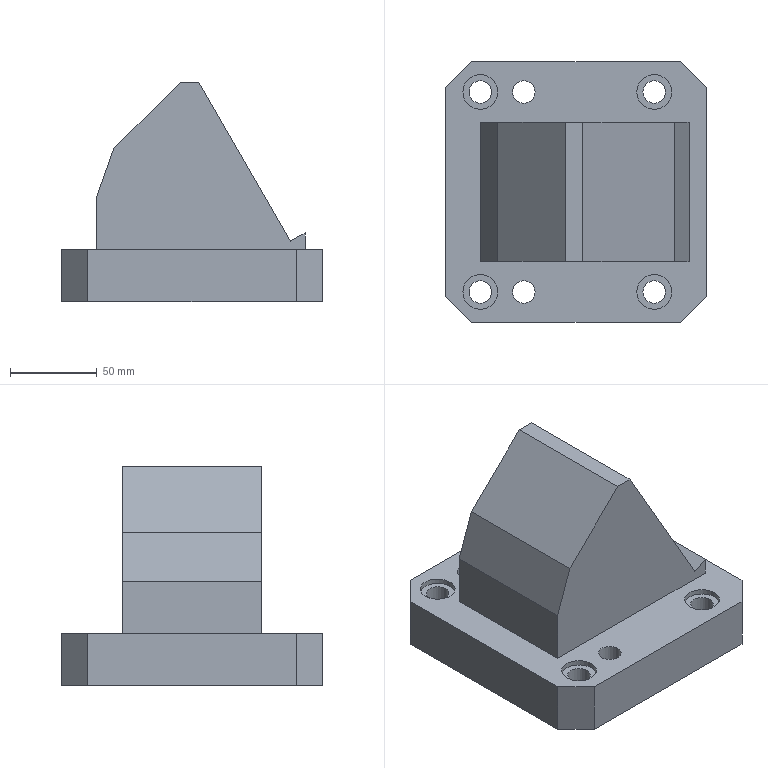Part | NX | features solid 2 | 1 solid | 42 faces | box 150 x 150 x 126.504 mm | volume 1190810 mm3 | plane 32 | cylinder 10 | commonest cylinder face diameters 13 x6 20 x4
STEP:
#1=CARTESIAN_POINT('',(5.,782.5,185.));
#2=VERTEX_POINT('',#1);
#3=CARTESIAN_POINT('',(-5.,782.5,185.));
#4=DIRECTION('',(0.,0.,1.));
#5=DIRECTION('',(1.,0.,0.));
#6=AXIS2_PLACEMENT_3D('',#3,#4,#5);
#7=CIRCLE('',#6,10.);
#8=EDGE_CURVE('',#2,#2,#7,.T.);
#9=ORIENTED_EDGE('',*,*,#8,.F.);
#10=EDGE_LOOP('',(#9));
#11=FACE_BOUND('',#10,.T.);
#12=CARTESIAN_POINT('',(-73.5,782.5,185.));
#13=VERTEX_POINT('',#12);
#14=CARTESIAN_POINT('',(-80.,782.5,185.));
#15=DIRECTION('',(0.,0.,1.));
#16=DIRECTION('',(1.,0.,0.));
#17=AXIS2_PLACEMENT_3D('',#14,#15,#16);
#18=CIRCLE('',#17,6.5);
#19=EDGE_CURVE('',#13,#13,#18,.T.);
#20=ORIENTED_EDGE('',*,*,#19,.F.);
#21=EDGE_LOOP('',(#20));
#22=FACE_BOUND('',#21,.T.);
#23=CARTESIAN_POINT('',(-95.,782.5,185.));
#24=VERTEX_POINT('',#23);
#25=CARTESIAN_POINT('',(-105.,782.5,185.));
#26=DIRECTION('',(0.,0.,1.));
#27=DIRECTION('',(1.,0.,0.));
#28=AXIS2_PLACEMENT_3D('',#25,#26,#27);
#29=CIRCLE('',#28,10.);
#30=EDGE_CURVE('',#24,#24,#29,.T.);
#31=ORIENTED_EDGE('',*,*,#30,.F.);
#32=EDGE_LOOP('',(#31));
#33=FACE_BOUND('',#32,.T.);
#34=CARTESIAN_POINT('',(-95.,667.5,185.));
#35=VERTEX_POINT('',#34);
#36=CARTESIAN_POINT('',(-105.,667.5,185.));
#37=DIRECTION('',(0.,0.,1.));
#38=DIRECTION('',(1.,0.,0.));
#39=AXIS2_PLACEMENT_3D('',#36,#37,#38);
#40=CIRCLE('',#39,10.);
#41=EDGE_CURVE('',#35,#35,#40,.T.);
#42=ORIENTED_EDGE('',*,*,#41,.F.);
#43=EDGE_LOOP('',(#42));
#44=FACE_BOUND('',#43,.T.);
#45=CARTESIAN_POINT('',(-73.5,667.5,185.));
#46=VERTEX_POINT('',#45);
#47=CARTESIAN_POINT('',(-80.,667.5,185.));
#48=DIRECTION('',(0.,0.,1.));
#49=DIRECTION('',(1.,0.,0.));
#50=AXIS2_PLACEMENT_3D('',#47,#48,#49);
#51=CIRCLE('',#50,6.5);
#52=EDGE_CURVE('',#46,#46,#51,.T.);
#53=ORIENTED_EDGE('',*,*,#52,.F.);
#54=EDGE_LOOP('',(#53));
#55=FACE_BOUND('',#54,.T.);
#56=CARTESIAN_POINT('',(5.,667.5,185.));
#57=VERTEX_POINT('',#56);
#58=CARTESIAN_POINT('',(-5.,667.5,185.));
#59=DIRECTION('',(0.,0.,1.));
#60=DIRECTION('',(1.,0.,0.));
#61=AXIS2_PLACEMENT_3D('',#58,#59,#60);
#62=CIRCLE('',#61,10.);
#63=EDGE_CURVE('',#57,#57,#62,.T.);
#64=ORIENTED_EDGE('',*,*,#63,.F.);
#65=EDGE_LOOP('',(#64));
#66=FACE_BOUND('',#65,.T.);
#67=CARTESIAN_POINT('',(-105.,685.,185.));
#68=VERTEX_POINT('',#67);
#69=CARTESIAN_POINT('',(15.,685.,185.));
#70=VERTEX_POINT('',#69);
#71=CARTESIAN_POINT('',(-125.,685.,185.));
#72=DIRECTION('',(1.,0.,0.));
#73=VECTOR('',#72,1000.);
#74=LINE('',#71,#73);
#75=EDGE_CURVE('',#68,#70,#74,.T.);
#76=ORIENTED_EDGE('',*,*,#75,.F.);
#77=CARTESIAN_POINT('',(-105.,765.,185.));
#78=VERTEX_POINT('',#77);
#79=CARTESIAN_POINT('',(-105.,685.,185.));
#80=DIRECTION('',(0.,1.,0.));
#81=VECTOR('',#80,1000.);
#82=LINE('',#79,#81);
#83=EDGE_CURVE('',#68,#78,#82,.T.);
#84=ORIENTED_EDGE('',*,*,#83,.T.);
#85=CARTESIAN_POINT('',(15.,765.,185.));
#86=VERTEX_POINT('',#85);
#87=CARTESIAN_POINT('',(-125.,765.,185.));
#88=DIRECTION('',(1.,0.,0.));
#89=VECTOR('',#88,1000.);
#90=LINE('',#87,#89);
#91=EDGE_CURVE('',#78,#86,#90,.T.);
#92=ORIENTED_EDGE('',*,*,#91,.T.);
#93=CARTESIAN_POINT('',(15.,685.,185.));
#94=DIRECTION('',(0.,1.,0.));
#95=VECTOR('',#94,1000.);
#96=LINE('',#93,#95);
#97=EDGE_CURVE('',#70,#86,#96,.T.);
#98=ORIENTED_EDGE('',*,*,#97,.F.);
#99=EDGE_LOOP('',(#76,#84,#92,#98));
#100=FACE_BOUND('',#99,.T.);
#101=CARTESIAN_POINT('',(-110.,800.,185.));
#102=VERTEX_POINT('',#101);
#103=CARTESIAN_POINT('',(10.,800.,185.));
#104=VERTEX_POINT('',#103);
#105=CARTESIAN_POINT('',(-125.,800.,185.));
#106=DIRECTION('',(1.,0.,0.));
#107=VECTOR('',#106,1000.);
#108=LINE('',#105,#107);
#109=EDGE_CURVE('',#102,#104,#108,.T.);
#110=ORIENTED_EDGE('',*,*,#109,.F.);
#111=CARTESIAN_POINT('',(-125.,785.,185.));
#112=VERTEX_POINT('',#111);
#113=CARTESIAN_POINT('',(-192.5,717.5,185.));
#114=DIRECTION('',(-0.7071,-0.7071,0.));
#115=VECTOR('',#114,1000.);
#116=LINE('',#113,#115);
#117=EDGE_CURVE('',#102,#112,#116,.T.);
#118=ORIENTED_EDGE('',*,*,#117,.T.);
#119=CARTESIAN_POINT('',(-125.,665.,185.));
#120=VERTEX_POINT('',#119);
#121=CARTESIAN_POINT('',(-125.,650.,185.));
#122=DIRECTION('',(0.,1.,0.));
#123=VECTOR('',#122,1000.);
#124=LINE('',#121,#123);
#125=EDGE_CURVE('',#120,#112,#124,.T.);
#126=ORIENTED_EDGE('',*,*,#125,.F.);
#127=CARTESIAN_POINT('',(-110.,650.,185.));
#128=VERTEX_POINT('',#127);
#129=CARTESIAN_POINT('',(-117.5,657.5,185.));
#130=DIRECTION('',(-0.7071,0.7071,0.));
#131=VECTOR('',#130,1000.);
#132=LINE('',#129,#131);
#133=EDGE_CURVE('',#120,#128,#132,.F.);
#134=ORIENTED_EDGE('',*,*,#133,.T.);
#135=CARTESIAN_POINT('',(10.,650.,185.));
#136=VERTEX_POINT('',#135);
#137=CARTESIAN_POINT('',(-125.,650.,185.));
#138=DIRECTION('',(1.,0.,0.));
#139=VECTOR('',#138,1000.);
#140=LINE('',#137,#139);
#141=EDGE_CURVE('',#128,#136,#140,.T.);
#142=ORIENTED_EDGE('',*,*,#141,.T.);
#143=CARTESIAN_POINT('',(25.,665.,185.));
#144=VERTEX_POINT('',#143);
#145=CARTESIAN_POINT('',(-57.5,582.5,185.));
#146=DIRECTION('',(0.7071,0.7071,0.));
#147=VECTOR('',#146,1000.);
#148=LINE('',#145,#147);
#149=EDGE_CURVE('',#136,#144,#148,.T.);
#150=ORIENTED_EDGE('',*,*,#149,.T.);
#151=CARTESIAN_POINT('',(25.,785.,185.));
#152=VERTEX_POINT('',#151);
#153=CARTESIAN_POINT('',(25.,650.,185.));
#154=DIRECTION('',(0.,1.,0.));
#155=VECTOR('',#154,1000.);
#156=LINE('',#153,#155);
#157=EDGE_CURVE('',#144,#152,#156,.T.);
#158=ORIENTED_EDGE('',*,*,#157,.T.);
#159=CARTESIAN_POINT('',(17.5,792.5,185.));
#160=DIRECTION('',(0.7071,-0.7071,0.));
#161=VECTOR('',#160,1000.);
#162=LINE('',#159,#161);
#163=EDGE_CURVE('',#152,#104,#162,.F.);
#164=ORIENTED_EDGE('',*,*,#163,.T.);
#165=EDGE_LOOP('',(#110,#118,#126,#134,#142,#150,#158,#164));
#166=FACE_BOUND('',#165,.T.);
#167=CARTESIAN_POINT('',(-125.,650.,185.));
#168=DIRECTION('',(0.,0.,1.));
#169=DIRECTION('',(1.,0.,0.));
#170=AXIS2_PLACEMENT_3D('',#167,#168,#169);
#171=PLANE('',#170);
#172=ADVANCED_FACE('',(#11,#22,#33,#44,#55,#66,#100,#166),#171,.T.);
#173=CARTESIAN_POINT('',(25.,665.,155.));
#174=VERTEX_POINT('',#173);
#175=CARTESIAN_POINT('',(25.,785.,155.));
#176=VERTEX_POINT('',#175);
#177=CARTESIAN_POINT('',(25.,650.,155.));
#178=DIRECTION('',(0.,1.,0.));
#179=VECTOR('',#178,1000.);
#180=LINE('',#177,#179);
#181=EDGE_CURVE('',#174,#176,#180,.T.);
#182=ORIENTED_EDGE('',*,*,#181,.T.);
#183=CARTESIAN_POINT('',(25.,785.,185.));
#184=DIRECTION('',(0.,0.,1.));
#185=VECTOR('',#184,1000.);
#186=LINE('',#183,#185);
#187=EDGE_CURVE('',#176,#152,#186,.T.);
#188=ORIENTED_EDGE('',*,*,#187,.T.);
#189=ORIENTED_EDGE('',*,*,#157,.F.);
#190=CARTESIAN_POINT('',(25.,665.,155.));
#191=DIRECTION('',(0.,0.,-1.));
#192=VECTOR('',#191,1000.);
#193=LINE('',#190,#192);
#194=EDGE_CURVE('',#144,#174,#193,.T.);
#195=ORIENTED_EDGE('',*,*,#194,.T.);
#196=EDGE_LOOP('',(#182,#188,#189,#195));
#197=FACE_BOUND('',#196,.T.);
#198=CARTESIAN_POINT('',(25.,650.,185.));
#199=DIRECTION('',(1.,0.,0.));
#200=DIRECTION('',(0.,0.,-1.));
#201=AXIS2_PLACEMENT_3D('',#198,#199,#200);
#202=PLANE('',#201);
#203=ADVANCED_FACE('',(#197),#202,.T.);
#204=CARTESIAN_POINT('',(-11.5,782.5,155.));
#205=VERTEX_POINT('',#204);
#206=CARTESIAN_POINT('',(-5.,782.5,155.));
#207=DIRECTION('',(0.,0.,-1.));
#208=DIRECTION('',(-1.,0.,0.));
#209=AXIS2_PLACEMENT_3D('',#206,#207,#208);
#210=CIRCLE('',#209,6.5);
#211=EDGE_CURVE('',#205,#205,#210,.T.);
#212=ORIENTED_EDGE('',*,*,#211,.F.);
#213=EDGE_LOOP('',(#212));
#214=FACE_BOUND('',#213,.T.);
#215=CARTESIAN_POINT('',(-86.5,782.5,155.));
#216=VERTEX_POINT('',#215);
#217=CARTESIAN_POINT('',(-80.,782.5,155.));
#218=DIRECTION('',(0.,0.,-1.));
#219=DIRECTION('',(-1.,0.,0.));
#220=AXIS2_PLACEMENT_3D('',#217,#218,#219);
#221=CIRCLE('',#220,6.5);
#222=EDGE_CURVE('',#216,#216,#221,.T.);
#223=ORIENTED_EDGE('',*,*,#222,.F.);
#224=EDGE_LOOP('',(#223));
#225=FACE_BOUND('',#224,.T.);
#226=CARTESIAN_POINT('',(-111.5,782.5,155.));
#227=VERTEX_POINT('',#226);
#228=CARTESIAN_POINT('',(-105.,782.5,155.));
#229=DIRECTION('',(0.,0.,-1.));
#230=DIRECTION('',(-1.,0.,0.));
#231=AXIS2_PLACEMENT_3D('',#228,#229,#230);
#232=CIRCLE('',#231,6.5);
#233=EDGE_CURVE('',#227,#227,#232,.T.);
#234=ORIENTED_EDGE('',*,*,#233,.F.);
#235=EDGE_LOOP('',(#234));
#236=FACE_BOUND('',#235,.T.);
#237=CARTESIAN_POINT('',(-111.5,667.5,155.));
#238=VERTEX_POINT('',#237);
#239=CARTESIAN_POINT('',(-105.,667.5,155.));
#240=DIRECTION('',(0.,0.,-1.));
#241=DIRECTION('',(-1.,0.,0.));
#242=AXIS2_PLACEMENT_3D('',#239,#240,#241);
#243=CIRCLE('',#242,6.5);
#244=EDGE_CURVE('',#238,#238,#243,.T.);
#245=ORIENTED_EDGE('',*,*,#244,.F.);
#246=EDGE_LOOP('',(#245));
#247=FACE_BOUND('',#246,.T.);
#248=CARTESIAN_POINT('',(-86.5,667.5,155.));
#249=VERTEX_POINT('',#248);
#250=CARTESIAN_POINT('',(-80.,667.5,155.));
#251=DIRECTION('',(0.,0.,-1.));
#252=DIRECTION('',(-1.,0.,0.));
#253=AXIS2_PLACEMENT_3D('',#250,#251,#252);
#254=CIRCLE('',#253,6.5);
#255=EDGE_CURVE('',#249,#249,#254,.T.);
#256=ORIENTED_EDGE('',*,*,#255,.F.);
#257=EDGE_LOOP('',(#256));
#258=FACE_BOUND('',#257,.T.);
#259=CARTESIAN_POINT('',(-11.5,667.5,155.));
#260=VERTEX_POINT('',#259);
#261=CARTESIAN_POINT('',(-5.,667.5,155.));
#262=DIRECTION('',(0.,0.,-1.));
#263=DIRECTION('',(-1.,0.,0.));
#264=AXIS2_PLACEMENT_3D('',#261,#262,#263);
#265=CIRCLE('',#264,6.5);
#266=EDGE_CURVE('',#260,#260,#265,.T.);
#267=ORIENTED_EDGE('',*,*,#266,.F.);
#268=EDGE_LOOP('',(#267));
#269=FACE_BOUND('',#268,.T.);
#270=CARTESIAN_POINT('',(-80.,735.,155.));
#271=VERTEX_POINT('',#270);
#272=CARTESIAN_POINT('',(-75.,740.,155.));
#273=VERTEX_POINT('',#272);
#274=CARTESIAN_POINT('',(-75.,740.,155.));
#275=DIRECTION('',(-0.7071,-0.7071,0.));
#276=VECTOR('',#275,1000.);
#277=LINE('',#274,#276);
#278=EDGE_CURVE('',#271,#273,#277,.F.);
#279=ORIENTED_EDGE('',*,*,#278,.F.);
#280=CARTESIAN_POINT('',(-80.,715.,155.));
#281=VERTEX_POINT('',#280);
#282=CARTESIAN_POINT('',(-80.,740.,155.));
#283=DIRECTION('',(0.,1.,0.));
#284=VECTOR('',#283,1000.);
#285=LINE('',#282,#284);
#286=EDGE_CURVE('',#271,#281,#285,.F.);
#287=ORIENTED_EDGE('',*,*,#286,.T.);
#288=CARTESIAN_POINT('',(-75.,710.,155.));
#289=VERTEX_POINT('',#288);
#290=CARTESIAN_POINT('',(-80.,715.,155.));
#291=DIRECTION('',(-0.7071,0.7071,0.));
#292=VECTOR('',#291,1000.);
#293=LINE('',#290,#292);
#294=EDGE_CURVE('',#289,#281,#293,.T.);
#295=ORIENTED_EDGE('',*,*,#294,.F.);
#296=CARTESIAN_POINT('',(-25.,710.,155.));
#297=VERTEX_POINT('',#296);
#298=CARTESIAN_POINT('',(10.,710.,155.));
#299=DIRECTION('',(-1.,0.,0.));
#300=VECTOR('',#299,1000.);
#301=LINE('',#298,#300);
#302=EDGE_CURVE('',#297,#289,#301,.T.);
#303=ORIENTED_EDGE('',*,*,#302,.F.);
#304=CARTESIAN_POINT('',(-20.,715.,155.));
#305=VERTEX_POINT('',#304);
#306=CARTESIAN_POINT('',(-25.,710.,155.));
#307=DIRECTION('',(0.7071,0.7071,0.));
#308=VECTOR('',#307,1000.);
#309=LINE('',#306,#308);
#310=EDGE_CURVE('',#305,#297,#309,.F.);
#311=ORIENTED_EDGE('',*,*,#310,.F.);
#312=CARTESIAN_POINT('',(-20.,735.,155.));
#313=VERTEX_POINT('',#312);
#314=CARTESIAN_POINT('',(-20.,740.,155.));
#315=DIRECTION('',(0.,-1.,0.));
#316=VECTOR('',#315,1000.);
#317=LINE('',#314,#316);
#318=EDGE_CURVE('',#313,#305,#317,.T.);
#319=ORIENTED_EDGE('',*,*,#318,.F.);
#320=CARTESIAN_POINT('',(-25.,740.,155.));
#321=VERTEX_POINT('',#320);
#322=CARTESIAN_POINT('',(-20.,735.,155.));
#323=DIRECTION('',(0.7071,-0.7071,0.));
#324=VECTOR('',#323,1000.);
#325=LINE('',#322,#324);
#326=EDGE_CURVE('',#321,#313,#325,.T.);
#327=ORIENTED_EDGE('',*,*,#326,.F.);
#328=CARTESIAN_POINT('',(10.,740.,155.));
#329=DIRECTION('',(-1.,0.,0.));
#330=VECTOR('',#329,1000.);
#331=LINE('',#328,#330);
#332=EDGE_CURVE('',#321,#273,#331,.T.);
#333=ORIENTED_EDGE('',*,*,#332,.T.);
#334=EDGE_LOOP('',(#279,#287,#295,#303,#311,#319,#327,#333));
#335=FACE_BOUND('',#334,.T.);
#336=CARTESIAN_POINT('',(-125.,665.,155.));
#337=VERTEX_POINT('',#336);
#338=CARTESIAN_POINT('',(-125.,785.,155.));
#339=VERTEX_POINT('',#338);
#340=CARTESIAN_POINT('',(-125.,650.,155.));
#341=DIRECTION('',(0.,1.,0.));
#342=VECTOR('',#341,1000.);
#343=LINE('',#340,#342);
#344=EDGE_CURVE('',#337,#339,#343,.T.);
#345=ORIENTED_EDGE('',*,*,#344,.T.);
#346=CARTESIAN_POINT('',(-110.,800.,155.));
#347=VERTEX_POINT('',#346);
#348=CARTESIAN_POINT('',(-117.5,792.5,155.));
#349=DIRECTION('',(0.7071,0.7071,0.));
#350=VECTOR('',#349,1000.);
#351=LINE('',#348,#350);
#352=EDGE_CURVE('',#339,#347,#351,.T.);
#353=ORIENTED_EDGE('',*,*,#352,.T.);
#354=CARTESIAN_POINT('',(10.,800.,155.));
#355=VERTEX_POINT('',#354);
#356=CARTESIAN_POINT('',(25.,800.,155.));
#357=DIRECTION('',(-1.,0.,0.));
#358=VECTOR('',#357,1000.);
#359=LINE('',#356,#358);
#360=EDGE_CURVE('',#355,#347,#359,.T.);
#361=ORIENTED_EDGE('',*,*,#360,.F.);
#362=CARTESIAN_POINT('',(92.5,717.5,155.));
#363=DIRECTION('',(-0.7071,0.7071,0.));
#364=VECTOR('',#363,1000.);
#365=LINE('',#362,#364);
#366=EDGE_CURVE('',#355,#176,#365,.F.);
#367=ORIENTED_EDGE('',*,*,#366,.T.);
#368=ORIENTED_EDGE('',*,*,#181,.F.);
#369=CARTESIAN_POINT('',(10.,650.,155.));
#370=VERTEX_POINT('',#369);
#371=CARTESIAN_POINT('',(17.5,657.5,155.));
#372=DIRECTION('',(-0.7071,-0.7071,0.));
#373=VECTOR('',#372,1000.);
#374=LINE('',#371,#373);
#375=EDGE_CURVE('',#174,#370,#374,.T.);
#376=ORIENTED_EDGE('',*,*,#375,.T.);
#377=CARTESIAN_POINT('',(-110.,650.,155.));
#378=VERTEX_POINT('',#377);
#379=CARTESIAN_POINT('',(25.,650.,155.));
#380=DIRECTION('',(-1.,0.,0.));
#381=VECTOR('',#380,1000.);
#382=LINE('',#379,#381);
#383=EDGE_CURVE('',#370,#378,#382,.T.);
#384=ORIENTED_EDGE('',*,*,#383,.T.);
#385=CARTESIAN_POINT('',(-42.5,582.5,155.));
#386=DIRECTION('',(0.7071,-0.7071,0.));
#387=VECTOR('',#386,1000.);
#388=LINE('',#385,#387);
#389=EDGE_CURVE('',#378,#337,#388,.F.);
#390=ORIENTED_EDGE('',*,*,#389,.T.);
#391=EDGE_LOOP('',(#345,#353,#361,#367,#368,#376,#384,#390));
#392=FACE_BOUND('',#391,.T.);
#393=CARTESIAN_POINT('',(25.,650.,155.));
#394=DIRECTION('',(0.,0.,-1.));
#395=DIRECTION('',(-1.,0.,0.));
#396=AXIS2_PLACEMENT_3D('',#393,#394,#395);
#397=PLANE('',#396);
#398=ADVANCED_FACE('',(#214,#225,#236,#247,#258,#269,#335,#392),#397,.T.);
#399=ORIENTED_EDGE('',*,*,#125,.T.);
#400=CARTESIAN_POINT('',(-125.,785.,155.));
#401=DIRECTION('',(0.,0.,-1.));
#402=VECTOR('',#401,1000.);
#403=LINE('',#400,#402);
#404=EDGE_CURVE('',#112,#339,#403,.T.);
#405=ORIENTED_EDGE('',*,*,#404,.T.);
#406=ORIENTED_EDGE('',*,*,#344,.F.);
#407=CARTESIAN_POINT('',(-125.,665.,185.));
#408=DIRECTION('',(0.,0.,1.));
#409=VECTOR('',#408,1000.);
#410=LINE('',#407,#409);
#411=EDGE_CURVE('',#337,#120,#410,.T.);
#412=ORIENTED_EDGE('',*,*,#411,.T.);
#413=EDGE_LOOP('',(#399,#405,#406,#412));
#414=FACE_BOUND('',#413,.T.);
#415=CARTESIAN_POINT('',(-125.,650.,185.));
#416=DIRECTION('',(1.,0.,0.));
#417=DIRECTION('',(0.,0.,-1.));
#418=AXIS2_PLACEMENT_3D('',#415,#416,#417);
#419=PLANE('',#418);
#420=ADVANCED_FACE('',(#414),#419,.F.);
#421=ORIENTED_EDGE('',*,*,#383,.F.);
#422=CARTESIAN_POINT('',(10.,650.,185.));
#423=DIRECTION('',(0.,0.,1.));
#424=VECTOR('',#423,1000.);
#425=LINE('',#422,#424);
#426=EDGE_CURVE('',#370,#136,#425,.T.);
#427=ORIENTED_EDGE('',*,*,#426,.T.);
#428=ORIENTED_EDGE('',*,*,#141,.F.);
#429=CARTESIAN_POINT('',(-110.,650.,185.));
#430=DIRECTION('',(0.,0.,-1.));
#431=VECTOR('',#430,1000.);
#432=LINE('',#429,#431);
#433=EDGE_CURVE('',#128,#378,#432,.T.);
#434=ORIENTED_EDGE('',*,*,#433,.T.);
#435=EDGE_LOOP('',(#421,#427,#428,#434));
#436=FACE_BOUND('',#435,.T.);
#437=CARTESIAN_POINT('',(25.,650.,185.));
#438=DIRECTION('',(0.,1.,0.));
#439=DIRECTION('',(0.,0.,1.));
#440=AXIS2_PLACEMENT_3D('',#437,#438,#439);
#441=PLANE('',#440);
#442=ADVANCED_FACE('',(#436),#441,.F.);
#443=ORIENTED_EDGE('',*,*,#360,.T.);
#444=CARTESIAN_POINT('',(-110.,800.,185.));
#445=DIRECTION('',(0.,0.,1.));
#446=VECTOR('',#445,1000.);
#447=LINE('',#444,#446);
#448=EDGE_CURVE('',#347,#102,#447,.T.);
#449=ORIENTED_EDGE('',*,*,#448,.T.);
#450=ORIENTED_EDGE('',*,*,#109,.T.);
#451=CARTESIAN_POINT('',(10.,800.,185.));
#452=DIRECTION('',(0.,0.,-1.));
#453=VECTOR('',#452,1000.);
#454=LINE('',#451,#453);
#455=EDGE_CURVE('',#104,#355,#454,.T.);
#456=ORIENTED_EDGE('',*,*,#455,.T.);
#457=EDGE_LOOP('',(#443,#449,#450,#456));
#458=FACE_BOUND('',#457,.T.);
#459=CARTESIAN_POINT('',(25.,800.,185.));
#460=DIRECTION('',(0.,1.,0.));
#461=DIRECTION('',(0.,0.,1.));
#462=AXIS2_PLACEMENT_3D('',#459,#460,#461);
#463=PLANE('',#462);
#464=ADVANCED_FACE('',(#458),#463,.T.);
#465=ORIENTED_EDGE('',*,*,#117,.F.);
#466=ORIENTED_EDGE('',*,*,#448,.F.);
#467=ORIENTED_EDGE('',*,*,#352,.F.);
#468=ORIENTED_EDGE('',*,*,#404,.F.);
#469=EDGE_LOOP('',(#465,#466,#467,#468));
#470=FACE_BOUND('',#469,.T.);
#471=CARTESIAN_POINT('',(-125.,785.,185.));
#472=DIRECTION('',(-0.7071,0.7071,0.));
#473=DIRECTION('',(-0.7071,-0.7071,0.));
#474=AXIS2_PLACEMENT_3D('',#471,#472,#473);
#475=PLANE('',#474);
#476=ADVANCED_FACE('',(#470),#475,.T.);
#477=ORIENTED_EDGE('',*,*,#163,.F.);
#478=ORIENTED_EDGE('',*,*,#187,.F.);
#479=ORIENTED_EDGE('',*,*,#366,.F.);
#480=ORIENTED_EDGE('',*,*,#455,.F.);
#481=EDGE_LOOP('',(#477,#478,#479,#480));
#482=FACE_BOUND('',#481,.T.);
#483=CARTESIAN_POINT('',(10.,800.,185.));
#484=DIRECTION('',(-0.7071,-0.7071,0.));
#485=DIRECTION('',(0.7071,-0.7071,0.));
#486=AXIS2_PLACEMENT_3D('',#483,#484,#485);
#487=PLANE('',#486);
#488=ADVANCED_FACE('',(#482),#487,.F.);
#489=ORIENTED_EDGE('',*,*,#149,.F.);
#490=ORIENTED_EDGE('',*,*,#426,.F.);
#491=ORIENTED_EDGE('',*,*,#375,.F.);
#492=ORIENTED_EDGE('',*,*,#194,.F.);
#493=EDGE_LOOP('',(#489,#490,#491,#492));
#494=FACE_BOUND('',#493,.T.);
#495=CARTESIAN_POINT('',(25.,665.,185.));
#496=DIRECTION('',(0.7071,-0.7071,0.));
#497=DIRECTION('',(0.7071,0.7071,0.));
#498=AXIS2_PLACEMENT_3D('',#495,#496,#497);
#499=PLANE('',#498);
#500=ADVANCED_FACE('',(#494),#499,.T.);
#501=ORIENTED_EDGE('',*,*,#133,.F.);
#502=ORIENTED_EDGE('',*,*,#411,.F.);
#503=ORIENTED_EDGE('',*,*,#389,.F.);
#504=ORIENTED_EDGE('',*,*,#433,.F.);
#505=EDGE_LOOP('',(#501,#502,#503,#504));
#506=FACE_BOUND('',#505,.T.);
#507=CARTESIAN_POINT('',(-110.,650.,185.));
#508=DIRECTION('',(0.7071,0.7071,0.));
#509=DIRECTION('',(-0.7071,0.7071,0.));
#510=AXIS2_PLACEMENT_3D('',#507,#508,#509);
#511=PLANE('',#510);
#512=ADVANCED_FACE('',(#506),#511,.F.);
#513=ORIENTED_EDGE('',*,*,#332,.F.);
#514=CARTESIAN_POINT('',(-25.,740.,165.));
#515=VERTEX_POINT('',#514);
#516=CARTESIAN_POINT('',(-25.,740.,155.));
#517=DIRECTION('',(0.,0.,1.));
#518=VECTOR('',#517,1000.);
#519=LINE('',#516,#518);
#520=EDGE_CURVE('',#515,#321,#519,.F.);
#521=ORIENTED_EDGE('',*,*,#520,.F.);
#522=CARTESIAN_POINT('',(-75.,740.,165.));
#523=VERTEX_POINT('',#522);
#524=CARTESIAN_POINT('',(10.,740.,165.));
#525=DIRECTION('',(1.,0.,0.));
#526=VECTOR('',#525,1000.);
#527=LINE('',#524,#526);
#528=EDGE_CURVE('',#515,#523,#527,.F.);
#529=ORIENTED_EDGE('',*,*,#528,.T.);
#530=CARTESIAN_POINT('',(-75.,740.,155.));
#531=DIRECTION('',(0.,0.,-1.));
#532=VECTOR('',#531,1000.);
#533=LINE('',#530,#532);
#534=EDGE_CURVE('',#273,#523,#533,.F.);
#535=ORIENTED_EDGE('',*,*,#534,.F.);
#536=EDGE_LOOP('',(#513,#521,#529,#535));
#537=FACE_BOUND('',#536,.T.);
#538=CARTESIAN_POINT('',(10.,740.,155.));
#539=DIRECTION('',(0.,1.,0.));
#540=DIRECTION('',(-1.,0.,0.));
#541=AXIS2_PLACEMENT_3D('',#538,#539,#540);
#542=PLANE('',#541);
#543=ADVANCED_FACE('',(#537),#542,.F.);
#544=ORIENTED_EDGE('',*,*,#318,.T.);
#545=CARTESIAN_POINT('',(-20.,715.,165.));
#546=VERTEX_POINT('',#545);
#547=CARTESIAN_POINT('',(-20.,715.,155.));
#548=DIRECTION('',(0.,0.,-1.));
#549=VECTOR('',#548,1000.);
#550=LINE('',#547,#549);
#551=EDGE_CURVE('',#546,#305,#550,.T.);
#552=ORIENTED_EDGE('',*,*,#551,.F.);
#553=CARTESIAN_POINT('',(-20.,735.,165.));
#554=VERTEX_POINT('',#553);
#555=CARTESIAN_POINT('',(-20.,740.,165.));
#556=DIRECTION('',(0.,-1.,0.));
#557=VECTOR('',#556,1000.);
#558=LINE('',#555,#557);
#559=EDGE_CURVE('',#554,#546,#558,.T.);
#560=ORIENTED_EDGE('',*,*,#559,.F.);
#561=CARTESIAN_POINT('',(-20.,735.,155.));
#562=DIRECTION('',(0.,0.,1.));
#563=VECTOR('',#562,1000.);
#564=LINE('',#561,#563);
#565=EDGE_CURVE('',#313,#554,#564,.T.);
#566=ORIENTED_EDGE('',*,*,#565,.F.);
#567=EDGE_LOOP('',(#544,#552,#560,#566));
#568=FACE_BOUND('',#567,.T.);
#569=CARTESIAN_POINT('',(-20.,740.,155.));
#570=DIRECTION('',(-1.,0.,0.));
#571=DIRECTION('',(0.,-1.,0.));
#572=AXIS2_PLACEMENT_3D('',#569,#570,#571);
#573=PLANE('',#572);
#574=ADVANCED_FACE('',(#568),#573,.T.);
#575=CARTESIAN_POINT('',(-25.,710.,165.));
#576=VERTEX_POINT('',#575);
#577=CARTESIAN_POINT('',(-75.,710.,165.));
#578=VERTEX_POINT('',#577);
#579=CARTESIAN_POINT('',(10.,710.,165.));
#580=DIRECTION('',(1.,0.,0.));
#581=VECTOR('',#580,1000.);
#582=LINE('',#579,#581);
#583=EDGE_CURVE('',#576,#578,#582,.F.);
#584=ORIENTED_EDGE('',*,*,#583,.F.);
#585=CARTESIAN_POINT('',(-25.,710.,155.));
#586=DIRECTION('',(0.,0.,1.));
#587=VECTOR('',#586,1000.);
#588=LINE('',#585,#587);
#589=EDGE_CURVE('',#297,#576,#588,.T.);
#590=ORIENTED_EDGE('',*,*,#589,.F.);
#591=ORIENTED_EDGE('',*,*,#302,.T.);
#592=CARTESIAN_POINT('',(-75.,710.,155.));
#593=DIRECTION('',(0.,0.,-1.));
#594=VECTOR('',#593,1000.);
#595=LINE('',#592,#594);
#596=EDGE_CURVE('',#578,#289,#595,.T.);
#597=ORIENTED_EDGE('',*,*,#596,.F.);
#598=EDGE_LOOP('',(#584,#590,#591,#597));
#599=FACE_BOUND('',#598,.T.);
#600=CARTESIAN_POINT('',(10.,710.,155.));
#601=DIRECTION('',(0.,1.,0.));
#602=DIRECTION('',(-1.,0.,0.));
#603=AXIS2_PLACEMENT_3D('',#600,#601,#602);
#604=PLANE('',#603);
#605=ADVANCED_FACE('',(#599),#604,.T.);
#606=CARTESIAN_POINT('',(-80.,735.,165.));
#607=VERTEX_POINT('',#606);
#608=CARTESIAN_POINT('',(-80.,715.,165.));
#609=VERTEX_POINT('',#608);
#610=CARTESIAN_POINT('',(-80.,740.,165.));
#611=DIRECTION('',(0.,1.,0.));
#612=VECTOR('',#611,1000.);
#613=LINE('',#610,#612);
#614=EDGE_CURVE('',#607,#609,#613,.F.);
#615=ORIENTED_EDGE('',*,*,#614,.T.);
#616=CARTESIAN_POINT('',(-80.,715.,155.));
#617=DIRECTION('',(0.,0.,-1.));
#618=VECTOR('',#617,1000.);
#619=LINE('',#616,#618);
#620=EDGE_CURVE('',#281,#609,#619,.F.);
#621=ORIENTED_EDGE('',*,*,#620,.F.);
#622=ORIENTED_EDGE('',*,*,#286,.F.);
#623=CARTESIAN_POINT('',(-80.,735.,155.));
#624=DIRECTION('',(0.,0.,1.));
#625=VECTOR('',#624,1000.);
#626=LINE('',#623,#625);
#627=EDGE_CURVE('',#607,#271,#626,.F.);
#628=ORIENTED_EDGE('',*,*,#627,.F.);
#629=EDGE_LOOP('',(#615,#621,#622,#628));
#630=FACE_BOUND('',#629,.T.);
#631=CARTESIAN_POINT('',(-80.,740.,155.));
#632=DIRECTION('',(-1.,0.,0.));
#633=DIRECTION('',(0.,-1.,0.));
#634=AXIS2_PLACEMENT_3D('',#631,#632,#633);
#635=PLANE('',#634);
#636=ADVANCED_FACE('',(#630),#635,.F.);
#637=ORIENTED_EDGE('',*,*,#528,.F.);
#638=CARTESIAN_POINT('',(-7.5,722.5,165.));
#639=DIRECTION('',(-0.7071,0.7071,0.));
#640=VECTOR('',#639,1000.);
#641=LINE('',#638,#640);
#642=EDGE_CURVE('',#554,#515,#641,.T.);
#643=ORIENTED_EDGE('',*,*,#642,.F.);
#644=ORIENTED_EDGE('',*,*,#559,.T.);
#645=CARTESIAN_POINT('',(7.5,742.5,165.));
#646=DIRECTION('',(-0.7071,-0.7071,0.));
#647=VECTOR('',#646,1000.);
#648=LINE('',#645,#647);
#649=EDGE_CURVE('',#576,#546,#648,.F.);
#650=ORIENTED_EDGE('',*,*,#649,.F.);
#651=ORIENTED_EDGE('',*,*,#583,.T.);
#652=CARTESIAN_POINT('',(-47.5,682.5,165.));
#653=DIRECTION('',(0.7071,-0.7071,0.));
#654=VECTOR('',#653,1000.);
#655=LINE('',#652,#654);
#656=EDGE_CURVE('',#609,#578,#655,.T.);
#657=ORIENTED_EDGE('',*,*,#656,.F.);
#658=ORIENTED_EDGE('',*,*,#614,.F.);
#659=CARTESIAN_POINT('',(-32.5,782.5,165.));
#660=DIRECTION('',(0.7071,0.7071,0.));
#661=VECTOR('',#660,1000.);
#662=LINE('',#659,#661);
#663=EDGE_CURVE('',#523,#607,#662,.F.);
#664=ORIENTED_EDGE('',*,*,#663,.F.);
#665=EDGE_LOOP('',(#637,#643,#644,#650,#651,#657,#658,#664));
#666=FACE_BOUND('',#665,.T.);
#667=CARTESIAN_POINT('',(10.,740.,165.));
#668=DIRECTION('',(0.,0.,1.));
#669=DIRECTION('',(1.,0.,0.));
#670=AXIS2_PLACEMENT_3D('',#667,#668,#669);
#671=PLANE('',#670);
#672=ADVANCED_FACE('',(#666),#671,.F.);
#673=ORIENTED_EDGE('',*,*,#278,.T.);
#674=ORIENTED_EDGE('',*,*,#534,.T.);
#675=ORIENTED_EDGE('',*,*,#663,.T.);
#676=ORIENTED_EDGE('',*,*,#627,.T.);
#677=EDGE_LOOP('',(#673,#674,#675,#676));
#678=FACE_BOUND('',#677,.T.);
#679=CARTESIAN_POINT('',(-75.,740.,155.));
#680=DIRECTION('',(0.7071,-0.7071,0.));
#681=DIRECTION('',(0.7071,0.7071,0.));
#682=AXIS2_PLACEMENT_3D('',#679,#680,#681);
#683=PLANE('',#682);
#684=ADVANCED_FACE('',(#678),#683,.T.);
#685=ORIENTED_EDGE('',*,*,#294,.T.);
#686=ORIENTED_EDGE('',*,*,#620,.T.);
#687=ORIENTED_EDGE('',*,*,#656,.T.);
#688=ORIENTED_EDGE('',*,*,#596,.T.);
#689=EDGE_LOOP('',(#685,#686,#687,#688));
#690=FACE_BOUND('',#689,.T.);
#691=CARTESIAN_POINT('',(-80.,715.,155.));
#692=DIRECTION('',(-0.7071,-0.7071,0.));
#693=DIRECTION('',(0.7071,-0.7071,0.));
#694=AXIS2_PLACEMENT_3D('',#691,#692,#693);
#695=PLANE('',#694);
#696=ADVANCED_FACE('',(#690),#695,.F.);
#697=ORIENTED_EDGE('',*,*,#326,.T.);
#698=ORIENTED_EDGE('',*,*,#565,.T.);
#699=ORIENTED_EDGE('',*,*,#642,.T.);
#700=ORIENTED_EDGE('',*,*,#520,.T.);
#701=EDGE_LOOP('',(#697,#698,#699,#700));
#702=FACE_BOUND('',#701,.T.);
#703=CARTESIAN_POINT('',(-20.,735.,155.));
#704=DIRECTION('',(0.7071,0.7071,0.));
#705=DIRECTION('',(-0.7071,0.7071,0.));
#706=AXIS2_PLACEMENT_3D('',#703,#704,#705);
#707=PLANE('',#706);
#708=ADVANCED_FACE('',(#702),#707,.F.);
#709=ORIENTED_EDGE('',*,*,#310,.T.);
#710=ORIENTED_EDGE('',*,*,#589,.T.);
#711=ORIENTED_EDGE('',*,*,#649,.T.);
#712=ORIENTED_EDGE('',*,*,#551,.T.);
#713=EDGE_LOOP('',(#709,#710,#711,#712));
#714=FACE_BOUND('',#713,.T.);
#715=CARTESIAN_POINT('',(-25.,710.,155.));
#716=DIRECTION('',(-0.7071,0.7071,0.));
#717=DIRECTION('',(-0.7071,-0.7071,0.));
#718=AXIS2_PLACEMENT_3D('',#715,#716,#717);
#719=PLANE('',#718);
#720=ADVANCED_FACE('',(#714),#719,.T.);
#721=CARTESIAN_POINT('',(-105.,765.,215.));
#722=VERTEX_POINT('',#721);
#723=CARTESIAN_POINT('',(-95.,765.,243.284));
#724=VERTEX_POINT('',#723);
#725=CARTESIAN_POINT('',(-105.,765.,215.));
#726=DIRECTION('',(0.3333,0.,0.9428));
#727=VECTOR('',#726,1000.);
#728=LINE('',#725,#727);
#729=EDGE_CURVE('',#722,#724,#728,.T.);
#730=ORIENTED_EDGE('',*,*,#729,.F.);
#731=CARTESIAN_POINT('',(-105.,685.,215.));
#732=VERTEX_POINT('',#731);
#733=CARTESIAN_POINT('',(-105.,685.,215.));
#734=DIRECTION('',(0.,1.,0.));
#735=VECTOR('',#734,1000.);
#736=LINE('',#733,#735);
#737=EDGE_CURVE('',#732,#722,#736,.T.);
#738=ORIENTED_EDGE('',*,*,#737,.F.);
#739=CARTESIAN_POINT('',(-95.,685.,243.284));
#740=VERTEX_POINT('',#739);
#741=CARTESIAN_POINT('',(-105.,685.,215.));
#742=DIRECTION('',(0.3333,0.,0.9428));
#743=VECTOR('',#742,1000.);
#744=LINE('',#741,#743);
#745=EDGE_CURVE('',#732,#740,#744,.T.);
#746=ORIENTED_EDGE('',*,*,#745,.T.);
#747=CARTESIAN_POINT('',(-95.,685.,243.284));
#748=DIRECTION('',(0.,1.,0.));
#749=VECTOR('',#748,1000.);
#750=LINE('',#747,#749);
#751=EDGE_CURVE('',#740,#724,#750,.T.);
#752=ORIENTED_EDGE('',*,*,#751,.T.);
#753=EDGE_LOOP('',(#730,#738,#746,#752));
#754=FACE_BOUND('',#753,.T.);
#755=CARTESIAN_POINT('',(-105.,685.,215.));
#756=DIRECTION('',(-0.9428,0.,0.3333));
#757=DIRECTION('',(0.3333,0.,0.9428));
#758=AXIS2_PLACEMENT_3D('',#755,#756,#757);
#759=PLANE('',#758);
#760=ADVANCED_FACE('',(#754),#759,.T.);
#761=CARTESIAN_POINT('',(-105.,765.,215.));
#762=DIRECTION('',(0.,0.,-1.));
#763=VECTOR('',#762,1000.);
#764=LINE('',#761,#763);
#765=EDGE_CURVE('',#722,#78,#764,.T.);
#766=ORIENTED_EDGE('',*,*,#765,.T.);
#767=ORIENTED_EDGE('',*,*,#83,.F.);
#768=CARTESIAN_POINT('',(-105.,685.,215.));
#769=DIRECTION('',(0.,0.,-1.));
#770=VECTOR('',#769,1000.);
#771=LINE('',#768,#770);
#772=EDGE_CURVE('',#732,#68,#771,.T.);
#773=ORIENTED_EDGE('',*,*,#772,.F.);
#774=ORIENTED_EDGE('',*,*,#737,.T.);
#775=EDGE_LOOP('',(#766,#767,#773,#774));
#776=FACE_BOUND('',#775,.T.);
#777=CARTESIAN_POINT('',(-105.,685.,215.));
#778=DIRECTION('',(1.,0.,0.));
#779=DIRECTION('',(0.,0.,-1.));
#780=AXIS2_PLACEMENT_3D('',#777,#778,#779);
#781=PLANE('',#780);
#782=ADVANCED_FACE('',(#776),#781,.F.);
#783=CARTESIAN_POINT('',(15.,765.,194.761));
#784=VERTEX_POINT('',#783);
#785=CARTESIAN_POINT('',(15.,765.,185.));
#786=DIRECTION('',(0.,0.,1.));
#787=VECTOR('',#786,1000.);
#788=LINE('',#785,#787);
#789=EDGE_CURVE('',#86,#784,#788,.T.);
#790=ORIENTED_EDGE('',*,*,#789,.T.);
#791=CARTESIAN_POINT('',(15.,685.,194.761));
#792=VERTEX_POINT('',#791);
#793=CARTESIAN_POINT('',(15.,685.,194.761));
#794=DIRECTION('',(0.,1.,0.));
#795=VECTOR('',#794,1000.);
#796=LINE('',#793,#795);
#797=EDGE_CURVE('',#792,#784,#796,.T.);
#798=ORIENTED_EDGE('',*,*,#797,.F.);
#799=CARTESIAN_POINT('',(15.,685.,185.));
#800=DIRECTION('',(0.,0.,1.));
#801=VECTOR('',#800,1000.);
#802=LINE('',#799,#801);
#803=EDGE_CURVE('',#70,#792,#802,.T.);
#804=ORIENTED_EDGE('',*,*,#803,.F.);
#805=ORIENTED_EDGE('',*,*,#97,.T.);
#806=EDGE_LOOP('',(#790,#798,#804,#805));
#807=FACE_BOUND('',#806,.T.);
#808=CARTESIAN_POINT('',(15.,685.,185.));
#809=DIRECTION('',(-1.,0.,0.));
#810=DIRECTION('',(0.,0.,1.));
#811=AXIS2_PLACEMENT_3D('',#808,#809,#810);
#812=PLANE('',#811);
#813=ADVANCED_FACE('',(#807),#812,.F.);
#814=CARTESIAN_POINT('',(6.753,765.,190.));
#815=VERTEX_POINT('',#814);
#816=CARTESIAN_POINT('',(6.753,765.,190.));
#817=DIRECTION('',(0.866,0.,0.5));
#818=VECTOR('',#817,1000.);
#819=LINE('',#816,#818);
#820=EDGE_CURVE('',#815,#784,#819,.T.);
#821=ORIENTED_EDGE('',*,*,#820,.F.);
#822=CARTESIAN_POINT('',(6.753,685.,190.));
#823=VERTEX_POINT('',#822);
#824=CARTESIAN_POINT('',(6.753,685.,190.));
#825=DIRECTION('',(0.,1.,0.));
#826=VECTOR('',#825,1000.);
#827=LINE('',#824,#826);
#828=EDGE_CURVE('',#823,#815,#827,.T.);
#829=ORIENTED_EDGE('',*,*,#828,.F.);
#830=CARTESIAN_POINT('',(6.753,685.,190.));
#831=DIRECTION('',(0.866,0.,0.5));
#832=VECTOR('',#831,1000.);
#833=LINE('',#830,#832);
#834=EDGE_CURVE('',#823,#792,#833,.T.);
#835=ORIENTED_EDGE('',*,*,#834,.T.);
#836=ORIENTED_EDGE('',*,*,#797,.T.);
#837=EDGE_LOOP('',(#821,#829,#835,#836));
#838=FACE_BOUND('',#837,.T.);
#839=CARTESIAN_POINT('',(6.753,685.,190.));
#840=DIRECTION('',(-0.5,0.,0.866));
#841=DIRECTION('',(0.866,0.,0.5));
#842=AXIS2_PLACEMENT_3D('',#839,#840,#841);
#843=PLANE('',#842);
#844=ADVANCED_FACE('',(#838),#843,.T.);
#845=CARTESIAN_POINT('',(-46.076,765.,281.504));
#846=VERTEX_POINT('',#845);
#847=CARTESIAN_POINT('',(-46.076,765.,281.504));
#848=DIRECTION('',(0.5,0.,-0.866));
#849=VECTOR('',#848,1000.);
#850=LINE('',#847,#849);
#851=EDGE_CURVE('',#846,#815,#850,.T.);
#852=ORIENTED_EDGE('',*,*,#851,.F.);
#853=CARTESIAN_POINT('',(-46.076,685.,281.504));
#854=VERTEX_POINT('',#853);
#855=CARTESIAN_POINT('',(-46.076,685.,281.504));
#856=DIRECTION('',(0.,1.,0.));
#857=VECTOR('',#856,1000.);
#858=LINE('',#855,#857);
#859=EDGE_CURVE('',#854,#846,#858,.T.);
#860=ORIENTED_EDGE('',*,*,#859,.F.);
#861=CARTESIAN_POINT('',(-46.076,685.,281.504));
#862=DIRECTION('',(0.5,0.,-0.866));
#863=VECTOR('',#862,1000.);
#864=LINE('',#861,#863);
#865=EDGE_CURVE('',#854,#823,#864,.T.);
#866=ORIENTED_EDGE('',*,*,#865,.T.);
#867=ORIENTED_EDGE('',*,*,#828,.T.);
#868=EDGE_LOOP('',(#852,#860,#866,#867));
#869=FACE_BOUND('',#868,.T.);
#870=CARTESIAN_POINT('',(-46.076,685.,281.504));
#871=DIRECTION('',(0.866,0.,0.5));
#872=DIRECTION('',(0.5,0.,-0.866));
#873=AXIS2_PLACEMENT_3D('',#870,#871,#872);
#874=PLANE('',#873);
#875=ADVANCED_FACE('',(#869),#874,.T.);
#876=CARTESIAN_POINT('',(-56.076,765.,281.504));
#877=VERTEX_POINT('',#876);
#878=CARTESIAN_POINT('',(-46.076,765.,281.504));
#879=DIRECTION('',(-1.,0.,0.));
#880=VECTOR('',#879,1000.);
#881=LINE('',#878,#880);
#882=EDGE_CURVE('',#846,#877,#881,.T.);
#883=ORIENTED_EDGE('',*,*,#882,.T.);
#884=CARTESIAN_POINT('',(-56.076,685.,281.504));
#885=VERTEX_POINT('',#884);
#886=CARTESIAN_POINT('',(-56.076,685.,281.504));
#887=DIRECTION('',(0.,1.,0.));
#888=VECTOR('',#887,1000.);
#889=LINE('',#886,#888);
#890=EDGE_CURVE('',#885,#877,#889,.T.);
#891=ORIENTED_EDGE('',*,*,#890,.F.);
#892=CARTESIAN_POINT('',(-46.076,685.,281.504));
#893=DIRECTION('',(-1.,0.,0.));
#894=VECTOR('',#893,1000.);
#895=LINE('',#892,#894);
#896=EDGE_CURVE('',#854,#885,#895,.T.);
#897=ORIENTED_EDGE('',*,*,#896,.F.);
#898=ORIENTED_EDGE('',*,*,#859,.T.);
#899=EDGE_LOOP('',(#883,#891,#897,#898));
#900=FACE_BOUND('',#899,.T.);
#901=CARTESIAN_POINT('',(-46.076,685.,281.504));
#902=DIRECTION('',(0.,0.,-1.));
#903=DIRECTION('',(-1.,0.,0.));
#904=AXIS2_PLACEMENT_3D('',#901,#902,#903);
#905=PLANE('',#904);
#906=ADVANCED_FACE('',(#900),#905,.F.);
#907=CARTESIAN_POINT('',(-56.076,765.,281.504));
#908=DIRECTION('',(-0.7135,0.,-0.7006));
#909=VECTOR('',#908,1000.);
#910=LINE('',#907,#909);
#911=EDGE_CURVE('',#877,#724,#910,.T.);
#912=ORIENTED_EDGE('',*,*,#911,.T.);
#913=ORIENTED_EDGE('',*,*,#751,.F.);
#914=CARTESIAN_POINT('',(-56.076,685.,281.504));
#915=DIRECTION('',(-0.7135,0.,-0.7006));
#916=VECTOR('',#915,1000.);
#917=LINE('',#914,#916);
#918=EDGE_CURVE('',#885,#740,#917,.T.);
#919=ORIENTED_EDGE('',*,*,#918,.F.);
#920=ORIENTED_EDGE('',*,*,#890,.T.);
#921=EDGE_LOOP('',(#912,#913,#919,#920));
#922=FACE_BOUND('',#921,.T.);
#923=CARTESIAN_POINT('',(-56.076,685.,281.504));
#924=DIRECTION('',(0.7006,0.,-0.7135));
#925=DIRECTION('',(-0.7135,0.,-0.7006));
#926=AXIS2_PLACEMENT_3D('',#923,#924,#925);
#927=PLANE('',#926);
#928=ADVANCED_FACE('',(#922),#927,.F.);
#929=ORIENTED_EDGE('',*,*,#745,.F.);
#930=ORIENTED_EDGE('',*,*,#772,.T.);
#931=ORIENTED_EDGE('',*,*,#75,.T.);
#932=ORIENTED_EDGE('',*,*,#803,.T.);
#933=ORIENTED_EDGE('',*,*,#834,.F.);
#934=ORIENTED_EDGE('',*,*,#865,.F.);
#935=ORIENTED_EDGE('',*,*,#896,.T.);
#936=ORIENTED_EDGE('',*,*,#918,.T.);
#937=EDGE_LOOP('',(#929,#930,#931,#932,#933,#934,#935,#936));
#938=FACE_BOUND('',#937,.T.);
#939=CARTESIAN_POINT('',(-45.816,685.,220.745));
#940=DIRECTION('',(0.,-1.,0.));
#941=DIRECTION('',(0.,0.,-1.));
#942=AXIS2_PLACEMENT_3D('',#939,#940,#941);
#943=PLANE('',#942);
#944=ADVANCED_FACE('',(#938),#943,.T.);
#945=ORIENTED_EDGE('',*,*,#729,.T.);
#946=ORIENTED_EDGE('',*,*,#911,.F.);
#947=ORIENTED_EDGE('',*,*,#882,.F.);
#948=ORIENTED_EDGE('',*,*,#851,.T.);
#949=ORIENTED_EDGE('',*,*,#820,.T.);
#950=ORIENTED_EDGE('',*,*,#789,.F.);
#951=ORIENTED_EDGE('',*,*,#91,.F.);
#952=ORIENTED_EDGE('',*,*,#765,.F.);
#953=EDGE_LOOP('',(#945,#946,#947,#948,#949,#950,#951,#952));
#954=FACE_BOUND('',#953,.T.);
#955=CARTESIAN_POINT('',(-45.816,765.,220.745));
#956=DIRECTION('',(0.,-1.,0.));
#957=DIRECTION('',(0.,0.,-1.));
#958=AXIS2_PLACEMENT_3D('',#955,#956,#957);
#959=PLANE('',#958);
#960=ADVANCED_FACE('',(#954),#959,.F.);
#961=ORIENTED_EDGE('',*,*,#63,.T.);
#962=EDGE_LOOP('',(#961));
#963=FACE_BOUND('',#962,.T.);
#964=CARTESIAN_POINT('',(5.,667.5,182.));
#965=VERTEX_POINT('',#964);
#966=CARTESIAN_POINT('',(-5.,667.5,182.));
#967=DIRECTION('',(0.,0.,-1.));
#968=DIRECTION('',(1.,0.,0.));
#969=AXIS2_PLACEMENT_3D('',#966,#967,#968);
#970=CIRCLE('',#969,10.);
#971=EDGE_CURVE('',#965,#965,#970,.T.);
#972=ORIENTED_EDGE('',*,*,#971,.T.);
#973=EDGE_LOOP('',(#972));
#974=FACE_BOUND('',#973,.T.);
#975=CARTESIAN_POINT('',(-5.,667.5,197.57));
#976=DIRECTION('',(0.,0.,-1.));
#977=DIRECTION('',(-1.,0.,0.));
#978=AXIS2_PLACEMENT_3D('',#975,#976,#977);
#979=CYLINDRICAL_SURFACE('',#978,10.);
#980=ADVANCED_FACE('',(#963,#974),#979,.F.);
#981=CARTESIAN_POINT('',(-11.5,667.5,182.));
#982=VERTEX_POINT('',#981);
#983=CARTESIAN_POINT('',(-5.,667.5,182.));
#984=DIRECTION('',(0.,0.,-1.));
#985=DIRECTION('',(-1.,0.,0.));
#986=AXIS2_PLACEMENT_3D('',#983,#984,#985);
#987=CIRCLE('',#986,6.5);
#988=EDGE_CURVE('',#982,#982,#987,.T.);
#989=ORIENTED_EDGE('',*,*,#988,.T.);
#990=EDGE_LOOP('',(#989));
#991=FACE_BOUND('',#990,.T.);
#992=ORIENTED_EDGE('',*,*,#971,.F.);
#993=EDGE_LOOP('',(#992));
#994=FACE_BOUND('',#993,.T.);
#995=CARTESIAN_POINT('',(-5.,667.5,182.));
#996=DIRECTION('',(0.,0.,-1.));
#997=DIRECTION('',(-1.,0.,0.));
#998=AXIS2_PLACEMENT_3D('',#995,#996,#997);
#999=PLANE('',#998);
#1000=ADVANCED_FACE('',(#991,#994),#999,.F.);
#1001=ORIENTED_EDGE('',*,*,#266,.T.);
#1002=EDGE_LOOP('',(#1001));
#1003=FACE_BOUND('',#1002,.T.);
#1004=ORIENTED_EDGE('',*,*,#988,.F.);
#1005=EDGE_LOOP('',(#1004));
#1006=FACE_BOUND('',#1005,.T.);
#1007=CARTESIAN_POINT('',(-5.,667.5,197.57));
#1008=DIRECTION('',(0.,0.,-1.));
#1009=DIRECTION('',(-1.,0.,0.));
#1010=AXIS2_PLACEMENT_3D('',#1007,#1008,#1009);
#1011=CYLINDRICAL_SURFACE('',#1010,6.5);
#1012=ADVANCED_FACE('',(#1003,#1006),#1011,.F.);
#1013=ORIENTED_EDGE('',*,*,#52,.T.);
#1014=EDGE_LOOP('',(#1013));
#1015=FACE_BOUND('',#1014,.T.);
#1016=ORIENTED_EDGE('',*,*,#255,.T.);
#1017=EDGE_LOOP('',(#1016));
#1018=FACE_BOUND('',#1017,.T.);
#1019=CARTESIAN_POINT('',(-80.,667.5,197.57));
#1020=DIRECTION('',(0.,0.,-1.));
#1021=DIRECTION('',(-1.,0.,0.));
#1022=AXIS2_PLACEMENT_3D('',#1019,#1020,#1021);
#1023=CYLINDRICAL_SURFACE('',#1022,6.5);
#1024=ADVANCED_FACE('',(#1015,#1018),#1023,.F.);
#1025=ORIENTED_EDGE('',*,*,#41,.T.);
#1026=EDGE_LOOP('',(#1025));
#1027=FACE_BOUND('',#1026,.T.);
#1028=CARTESIAN_POINT('',(-95.,667.5,182.));
#1029=VERTEX_POINT('',#1028);
#1030=CARTESIAN_POINT('',(-105.,667.5,182.));
#1031=DIRECTION('',(0.,0.,-1.));
#1032=DIRECTION('',(1.,0.,0.));
#1033=AXIS2_PLACEMENT_3D('',#1030,#1031,#1032);
#1034=CIRCLE('',#1033,10.);
#1035=EDGE_CURVE('',#1029,#1029,#1034,.T.);
#1036=ORIENTED_EDGE('',*,*,#1035,.T.);
#1037=EDGE_LOOP('',(#1036));
#1038=FACE_BOUND('',#1037,.T.);
#1039=CARTESIAN_POINT('',(-105.,667.5,197.57));
#1040=DIRECTION('',(0.,0.,-1.));
#1041=DIRECTION('',(-1.,0.,0.));
#1042=AXIS2_PLACEMENT_3D('',#1039,#1040,#1041);
#1043=CYLINDRICAL_SURFACE('',#1042,10.);
#1044=ADVANCED_FACE('',(#1027,#1038),#1043,.F.);
#1045=CARTESIAN_POINT('',(-111.5,667.5,182.));
#1046=VERTEX_POINT('',#1045);
#1047=CARTESIAN_POINT('',(-105.,667.5,182.));
#1048=DIRECTION('',(0.,0.,-1.));
#1049=DIRECTION('',(-1.,0.,0.));
#1050=AXIS2_PLACEMENT_3D('',#1047,#1048,#1049);
#1051=CIRCLE('',#1050,6.5);
#1052=EDGE_CURVE('',#1046,#1046,#1051,.T.);
#1053=ORIENTED_EDGE('',*,*,#1052,.T.);
#1054=EDGE_LOOP('',(#1053));
#1055=FACE_BOUND('',#1054,.T.);
#1056=ORIENTED_EDGE('',*,*,#1035,.F.);
#1057=EDGE_LOOP('',(#1056));
#1058=FACE_BOUND('',#1057,.T.);
#1059=CARTESIAN_POINT('',(-105.,667.5,182.));
#1060=DIRECTION('',(0.,0.,-1.));
#1061=DIRECTION('',(-1.,0.,0.));
#1062=AXIS2_PLACEMENT_3D('',#1059,#1060,#1061);
#1063=PLANE('',#1062);
#1064=ADVANCED_FACE('',(#1055,#1058),#1063,.F.);
#1065=ORIENTED_EDGE('',*,*,#244,.T.);
#1066=EDGE_LOOP('',(#1065));
#1067=FACE_BOUND('',#1066,.T.);
#1068=ORIENTED_EDGE('',*,*,#1052,.F.);
#1069=EDGE_LOOP('',(#1068));
#1070=FACE_BOUND('',#1069,.T.);
#1071=CARTESIAN_POINT('',(-105.,667.5,197.57));
#1072=DIRECTION('',(0.,0.,-1.));
#1073=DIRECTION('',(-1.,0.,0.));
#1074=AXIS2_PLACEMENT_3D('',#1071,#1072,#1073);
#1075=CYLINDRICAL_SURFACE('',#1074,6.5);
#1076=ADVANCED_FACE('',(#1067,#1070),#1075,.F.);
#1077=ORIENTED_EDGE('',*,*,#30,.T.);
#1078=EDGE_LOOP('',(#1077));
#1079=FACE_BOUND('',#1078,.T.);
#1080=CARTESIAN_POINT('',(-95.,782.5,182.));
#1081=VERTEX_POINT('',#1080);
#1082=CARTESIAN_POINT('',(-105.,782.5,182.));
#1083=DIRECTION('',(0.,0.,-1.));
#1084=DIRECTION('',(1.,0.,0.));
#1085=AXIS2_PLACEMENT_3D('',#1082,#1083,#1084);
#1086=CIRCLE('',#1085,10.);
#1087=EDGE_CURVE('',#1081,#1081,#1086,.T.);
#1088=ORIENTED_EDGE('',*,*,#1087,.T.);
#1089=EDGE_LOOP('',(#1088));
#1090=FACE_BOUND('',#1089,.T.);
#1091=CARTESIAN_POINT('',(-105.,782.5,197.57));
#1092=DIRECTION('',(0.,0.,-1.));
#1093=DIRECTION('',(-1.,0.,0.));
#1094=AXIS2_PLACEMENT_3D('',#1091,#1092,#1093);
#1095=CYLINDRICAL_SURFACE('',#1094,10.);
#1096=ADVANCED_FACE('',(#1079,#1090),#1095,.F.);
#1097=CARTESIAN_POINT('',(-111.5,782.5,182.));
#1098=VERTEX_POINT('',#1097);
#1099=CARTESIAN_POINT('',(-105.,782.5,182.));
#1100=DIRECTION('',(0.,0.,-1.));
#1101=DIRECTION('',(-1.,0.,0.));
#1102=AXIS2_PLACEMENT_3D('',#1099,#1100,#1101);
#1103=CIRCLE('',#1102,6.5);
#1104=EDGE_CURVE('',#1098,#1098,#1103,.T.);
#1105=ORIENTED_EDGE('',*,*,#1104,.T.);
#1106=EDGE_LOOP('',(#1105));
#1107=FACE_BOUND('',#1106,.T.);
#1108=ORIENTED_EDGE('',*,*,#1087,.F.);
#1109=EDGE_LOOP('',(#1108));
#1110=FACE_BOUND('',#1109,.T.);
#1111=CARTESIAN_POINT('',(-105.,782.5,182.));
#1112=DIRECTION('',(0.,0.,-1.));
#1113=DIRECTION('',(-1.,0.,0.));
#1114=AXIS2_PLACEMENT_3D('',#1111,#1112,#1113);
#1115=PLANE('',#1114);
#1116=ADVANCED_FACE('',(#1107,#1110),#1115,.F.);
#1117=ORIENTED_EDGE('',*,*,#233,.T.);
#1118=EDGE_LOOP('',(#1117));
#1119=FACE_BOUND('',#1118,.T.);
#1120=ORIENTED_EDGE('',*,*,#1104,.F.);
#1121=EDGE_LOOP('',(#1120));
#1122=FACE_BOUND('',#1121,.T.);
#1123=CARTESIAN_POINT('',(-105.,782.5,197.57));
#1124=DIRECTION('',(0.,0.,-1.));
#1125=DIRECTION('',(-1.,0.,0.));
#1126=AXIS2_PLACEMENT_3D('',#1123,#1124,#1125);
#1127=CYLINDRICAL_SURFACE('',#1126,6.5);
#1128=ADVANCED_FACE('',(#1119,#1122),#1127,.F.);
#1129=ORIENTED_EDGE('',*,*,#19,.T.);
#1130=EDGE_LOOP('',(#1129));
#1131=FACE_BOUND('',#1130,.T.);
#1132=ORIENTED_EDGE('',*,*,#222,.T.);
#1133=EDGE_LOOP('',(#1132));
#1134=FACE_BOUND('',#1133,.T.);
#1135=CARTESIAN_POINT('',(-80.,782.5,197.57));
#1136=DIRECTION('',(0.,0.,-1.));
#1137=DIRECTION('',(-1.,0.,0.));
#1138=AXIS2_PLACEMENT_3D('',#1135,#1136,#1137);
#1139=CYLINDRICAL_SURFACE('',#1138,6.5);
#1140=ADVANCED_FACE('',(#1131,#1134),#1139,.F.);
#1141=ORIENTED_EDGE('',*,*,#8,.T.);
#1142=EDGE_LOOP('',(#1141));
#1143=FACE_BOUND('',#1142,.T.);
#1144=CARTESIAN_POINT('',(5.,782.5,182.));
#1145=VERTEX_POINT('',#1144);
#1146=CARTESIAN_POINT('',(-5.,782.5,182.));
#1147=DIRECTION('',(0.,0.,-1.));
#1148=DIRECTION('',(1.,0.,0.));
#1149=AXIS2_PLACEMENT_3D('',#1146,#1147,#1148);
#1150=CIRCLE('',#1149,10.);
#1151=EDGE_CURVE('',#1145,#1145,#1150,.T.);
#1152=ORIENTED_EDGE('',*,*,#1151,.T.);
#1153=EDGE_LOOP('',(#1152));
#1154=FACE_BOUND('',#1153,.T.);
#1155=CARTESIAN_POINT('',(-5.,782.5,197.57));
#1156=DIRECTION('',(0.,0.,-1.));
#1157=DIRECTION('',(-1.,0.,0.));
#1158=AXIS2_PLACEMENT_3D('',#1155,#1156,#1157);
#1159=CYLINDRICAL_SURFACE('',#1158,10.);
#1160=ADVANCED_FACE('',(#1143,#1154),#1159,.F.);
#1161=CARTESIAN_POINT('',(-11.5,782.5,182.));
#1162=VERTEX_POINT('',#1161);
#1163=CARTESIAN_POINT('',(-5.,782.5,182.));
#1164=DIRECTION('',(0.,0.,-1.));
#1165=DIRECTION('',(-1.,0.,0.));
#1166=AXIS2_PLACEMENT_3D('',#1163,#1164,#1165);
#1167=CIRCLE('',#1166,6.5);
#1168=EDGE_CURVE('',#1162,#1162,#1167,.T.);
#1169=ORIENTED_EDGE('',*,*,#1168,.T.);
#1170=EDGE_LOOP('',(#1169));
#1171=FACE_BOUND('',#1170,.T.);
#1172=ORIENTED_EDGE('',*,*,#1151,.F.);
#1173=EDGE_LOOP('',(#1172));
#1174=FACE_BOUND('',#1173,.T.);
#1175=CARTESIAN_POINT('',(-5.,782.5,182.));
#1176=DIRECTION('',(0.,0.,-1.));
#1177=DIRECTION('',(-1.,0.,0.));
#1178=AXIS2_PLACEMENT_3D('',#1175,#1176,#1177);
#1179=PLANE('',#1178);
#1180=ADVANCED_FACE('',(#1171,#1174),#1179,.F.);
#1181=ORIENTED_EDGE('',*,*,#211,.T.);
#1182=EDGE_LOOP('',(#1181));
#1183=FACE_BOUND('',#1182,.T.);
#1184=ORIENTED_EDGE('',*,*,#1168,.F.);
#1185=EDGE_LOOP('',(#1184));
#1186=FACE_BOUND('',#1185,.T.);
#1187=CARTESIAN_POINT('',(-5.,782.5,197.57));
#1188=DIRECTION('',(0.,0.,-1.));
#1189=DIRECTION('',(-1.,0.,0.));
#1190=AXIS2_PLACEMENT_3D('',#1187,#1188,#1189);
#1191=CYLINDRICAL_SURFACE('',#1190,6.5);
#1192=ADVANCED_FACE('',(#1183,#1186),#1191,.F.);
#1193=CLOSED_SHELL('',(#172,#203,#398,#420,#442,#464,#476,#488,#500,#512,#543,#574,#605,#636,#672,#684,#696,#708,#720,#760,#782,#813,#844,#875,#906,#928,#944,#960,#980,#1000,#1012,#1024,#1044,#1064,#1076,#1096,#1116,#1128,#1140,#1160,#1180,#1192));
#1194=MANIFOLD_SOLID_BREP('',#1193);
#1195=(LENGTH_UNIT()NAMED_UNIT(*)SI_UNIT(.MILLI.,.METRE.));
#1196=UNCERTAINTY_MEASURE_WITH_UNIT(LENGTH_MEASURE(0.00001),#1195,'','');
#1197=(NAMED_UNIT(*)PLANE_ANGLE_UNIT()SI_UNIT($,.RADIAN.));
#1198=(NAMED_UNIT(*)SI_UNIT($,.STERADIAN.)SOLID_ANGLE_UNIT());
#1199=(GEOMETRIC_REPRESENTATION_CONTEXT(3)GLOBAL_UNCERTAINTY_ASSIGNED_CONTEXT((#1196))GLOBAL_UNIT_ASSIGNED_CONTEXT((#1195,#1197,#1198))REPRESENTATION_CONTEXT('',''));
#1200=ADVANCED_BREP_SHAPE_REPRESENTATION('',(#1194),#1199);